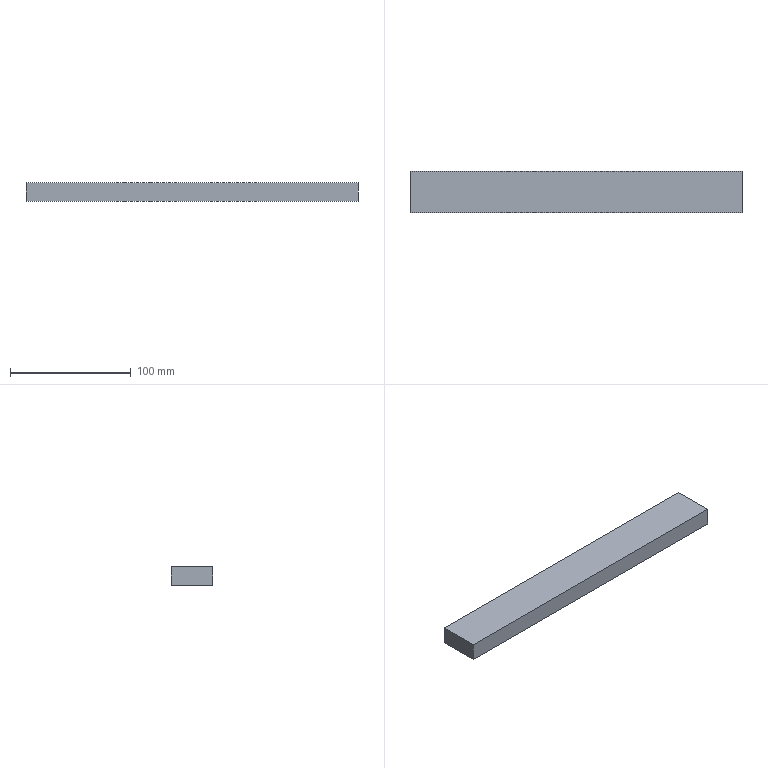Part | SolidWorks | features Extrusion 1 | 1 solid | 6 faces | box 275 x 34 x 15 mm | volume 140250 mm3 | plane 6
STEP:
#1=CARTESIAN_POINT('',(137.5,-17.,0.));
#2=VERTEX_POINT('',#1);
#3=CARTESIAN_POINT('',(137.5,17.,0.));
#4=VERTEX_POINT('',#3);
#5=CARTESIAN_POINT('',(137.5,-17.,0.));
#6=DIRECTION('',(0.,1.,0.));
#7=VECTOR('',#6,1000.);
#8=LINE('',#5,#7);
#9=EDGE_CURVE('',#2,#4,#8,.T.);
#10=ORIENTED_EDGE('',*,*,#9,.T.);
#11=CARTESIAN_POINT('',(137.5,17.,15.));
#12=VERTEX_POINT('',#11);
#13=CARTESIAN_POINT('',(137.5,17.,15.));
#14=DIRECTION('',(0.,0.,-1.));
#15=VECTOR('',#14,1000.);
#16=LINE('',#13,#15);
#17=EDGE_CURVE('',#12,#4,#16,.T.);
#18=ORIENTED_EDGE('',*,*,#17,.F.);
#19=CARTESIAN_POINT('',(137.5,-17.,15.));
#20=VERTEX_POINT('',#19);
#21=CARTESIAN_POINT('',(137.5,-17.,15.));
#22=DIRECTION('',(0.,1.,0.));
#23=VECTOR('',#22,1000.);
#24=LINE('',#21,#23);
#25=EDGE_CURVE('',#20,#12,#24,.T.);
#26=ORIENTED_EDGE('',*,*,#25,.F.);
#27=CARTESIAN_POINT('',(137.5,-17.,15.));
#28=DIRECTION('',(0.,0.,-1.));
#29=VECTOR('',#28,1000.);
#30=LINE('',#27,#29);
#31=EDGE_CURVE('',#20,#2,#30,.T.);
#32=ORIENTED_EDGE('',*,*,#31,.T.);
#33=EDGE_LOOP('',(#10,#18,#26,#32));
#34=FACE_OUTER_BOUND('',#33,.T.);
#35=CARTESIAN_POINT('',(137.5,-17.,15.));
#36=DIRECTION('',(-1.,0.,0.));
#37=DIRECTION('',(0.,0.,1.));
#38=AXIS2_PLACEMENT_3D('',#35,#36,#37);
#39=PLANE('',#38);
#40=ADVANCED_FACE('',(#34),#39,.F.);
#41=CARTESIAN_POINT('',(-137.5,17.,0.));
#42=VERTEX_POINT('',#41);
#43=CARTESIAN_POINT('',(-137.5,17.,0.));
#44=DIRECTION('',(-1.,0.,0.));
#45=VECTOR('',#44,1000.);
#46=LINE('',#43,#45);
#47=EDGE_CURVE('',#4,#42,#46,.T.);
#48=ORIENTED_EDGE('',*,*,#47,.T.);
#49=CARTESIAN_POINT('',(-137.5,17.,15.));
#50=VERTEX_POINT('',#49);
#51=CARTESIAN_POINT('',(-137.5,17.,15.));
#52=DIRECTION('',(0.,0.,-1.));
#53=VECTOR('',#52,1000.);
#54=LINE('',#51,#53);
#55=EDGE_CURVE('',#50,#42,#54,.T.);
#56=ORIENTED_EDGE('',*,*,#55,.F.);
#57=CARTESIAN_POINT('',(-137.5,17.,15.));
#58=DIRECTION('',(-1.,0.,0.));
#59=VECTOR('',#58,1000.);
#60=LINE('',#57,#59);
#61=EDGE_CURVE('',#12,#50,#60,.T.);
#62=ORIENTED_EDGE('',*,*,#61,.F.);
#63=ORIENTED_EDGE('',*,*,#17,.T.);
#64=EDGE_LOOP('',(#48,#56,#62,#63));
#65=FACE_OUTER_BOUND('',#64,.T.);
#66=CARTESIAN_POINT('',(-137.5,17.,15.));
#67=DIRECTION('',(0.,-1.,0.));
#68=DIRECTION('',(0.,0.,-1.));
#69=AXIS2_PLACEMENT_3D('',#66,#67,#68);
#70=PLANE('',#69);
#71=ADVANCED_FACE('',(#65),#70,.F.);
#72=CARTESIAN_POINT('',(-137.5,-17.,0.));
#73=VERTEX_POINT('',#72);
#74=CARTESIAN_POINT('',(-137.5,-17.,0.));
#75=DIRECTION('',(0.,-1.,0.));
#76=VECTOR('',#75,1000.);
#77=LINE('',#74,#76);
#78=EDGE_CURVE('',#42,#73,#77,.T.);
#79=ORIENTED_EDGE('',*,*,#78,.T.);
#80=CARTESIAN_POINT('',(-137.5,-17.,15.));
#81=VERTEX_POINT('',#80);
#82=CARTESIAN_POINT('',(-137.5,-17.,15.));
#83=DIRECTION('',(0.,0.,-1.));
#84=VECTOR('',#83,1000.);
#85=LINE('',#82,#84);
#86=EDGE_CURVE('',#81,#73,#85,.T.);
#87=ORIENTED_EDGE('',*,*,#86,.F.);
#88=CARTESIAN_POINT('',(-137.5,-17.,15.));
#89=DIRECTION('',(0.,-1.,0.));
#90=VECTOR('',#89,1000.);
#91=LINE('',#88,#90);
#92=EDGE_CURVE('',#50,#81,#91,.T.);
#93=ORIENTED_EDGE('',*,*,#92,.F.);
#94=ORIENTED_EDGE('',*,*,#55,.T.);
#95=EDGE_LOOP('',(#79,#87,#93,#94));
#96=FACE_OUTER_BOUND('',#95,.T.);
#97=CARTESIAN_POINT('',(-137.5,-17.,15.));
#98=DIRECTION('',(1.,0.,0.));
#99=DIRECTION('',(0.,0.,-1.));
#100=AXIS2_PLACEMENT_3D('',#97,#98,#99);
#101=PLANE('',#100);
#102=ADVANCED_FACE('',(#96),#101,.F.);
#103=CARTESIAN_POINT('',(-137.5,-17.,0.));
#104=DIRECTION('',(1.,0.,0.));
#105=VECTOR('',#104,1000.);
#106=LINE('',#103,#105);
#107=EDGE_CURVE('',#73,#2,#106,.T.);
#108=ORIENTED_EDGE('',*,*,#107,.T.);
#109=ORIENTED_EDGE('',*,*,#31,.F.);
#110=CARTESIAN_POINT('',(-137.5,-17.,15.));
#111=DIRECTION('',(1.,0.,0.));
#112=VECTOR('',#111,1000.);
#113=LINE('',#110,#112);
#114=EDGE_CURVE('',#81,#20,#113,.T.);
#115=ORIENTED_EDGE('',*,*,#114,.F.);
#116=ORIENTED_EDGE('',*,*,#86,.T.);
#117=EDGE_LOOP('',(#108,#109,#115,#116));
#118=FACE_OUTER_BOUND('',#117,.T.);
#119=CARTESIAN_POINT('',(-137.5,-17.,15.));
#120=DIRECTION('',(0.,1.,0.));
#121=DIRECTION('',(0.,0.,1.));
#122=AXIS2_PLACEMENT_3D('',#119,#120,#121);
#123=PLANE('',#122);
#124=ADVANCED_FACE('',(#118),#123,.F.);
#125=ORIENTED_EDGE('',*,*,#25,.T.);
#126=ORIENTED_EDGE('',*,*,#61,.T.);
#127=ORIENTED_EDGE('',*,*,#92,.T.);
#128=ORIENTED_EDGE('',*,*,#114,.T.);
#129=EDGE_LOOP('',(#125,#126,#127,#128));
#130=FACE_OUTER_BOUND('',#129,.T.);
#131=CARTESIAN_POINT('',(0.,0.,15.));
#132=DIRECTION('',(0.,0.,-1.));
#133=DIRECTION('',(-1.,0.,0.));
#134=AXIS2_PLACEMENT_3D('',#131,#132,#133);
#135=PLANE('',#134);
#136=ADVANCED_FACE('',(#130),#135,.F.);
#137=ORIENTED_EDGE('',*,*,#9,.F.);
#138=ORIENTED_EDGE('',*,*,#107,.F.);
#139=ORIENTED_EDGE('',*,*,#78,.F.);
#140=ORIENTED_EDGE('',*,*,#47,.F.);
#141=EDGE_LOOP('',(#137,#138,#139,#140));
#142=FACE_OUTER_BOUND('',#141,.T.);
#143=CARTESIAN_POINT('',(0.,0.,0.));
#144=DIRECTION('',(0.,0.,-1.));
#145=DIRECTION('',(-1.,0.,0.));
#146=AXIS2_PLACEMENT_3D('',#143,#144,#145);
#147=PLANE('',#146);
#148=ADVANCED_FACE('',(#142),#147,.T.);
#149=CLOSED_SHELL('',(#40,#71,#102,#124,#136,#148));
#150=MANIFOLD_SOLID_BREP('',#149);
#151=CARTESIAN_POINT('',(0.,0.,0.));
#152=DIRECTION('',(0.,0.,1.));
#153=DIRECTION('',(1.,0.,0.));
#154=AXIS2_PLACEMENT_3D('',#151,#152,#153);
#155=(LENGTH_UNIT()NAMED_UNIT(*)SI_UNIT(.MILLI.,.METRE.));
#156=UNCERTAINTY_MEASURE_WITH_UNIT(LENGTH_MEASURE(0.00001),#155,'','');
#157=(NAMED_UNIT(*)PLANE_ANGLE_UNIT()SI_UNIT($,.RADIAN.));
#158=(NAMED_UNIT(*)SI_UNIT($,.STERADIAN.)SOLID_ANGLE_UNIT());
#159=(GEOMETRIC_REPRESENTATION_CONTEXT(3)GLOBAL_UNCERTAINTY_ASSIGNED_CONTEXT((#156))GLOBAL_UNIT_ASSIGNED_CONTEXT((#155,#157,#158))REPRESENTATION_CONTEXT('',''));
#160=ADVANCED_BREP_SHAPE_REPRESENTATION('',(#150,#154),#159);